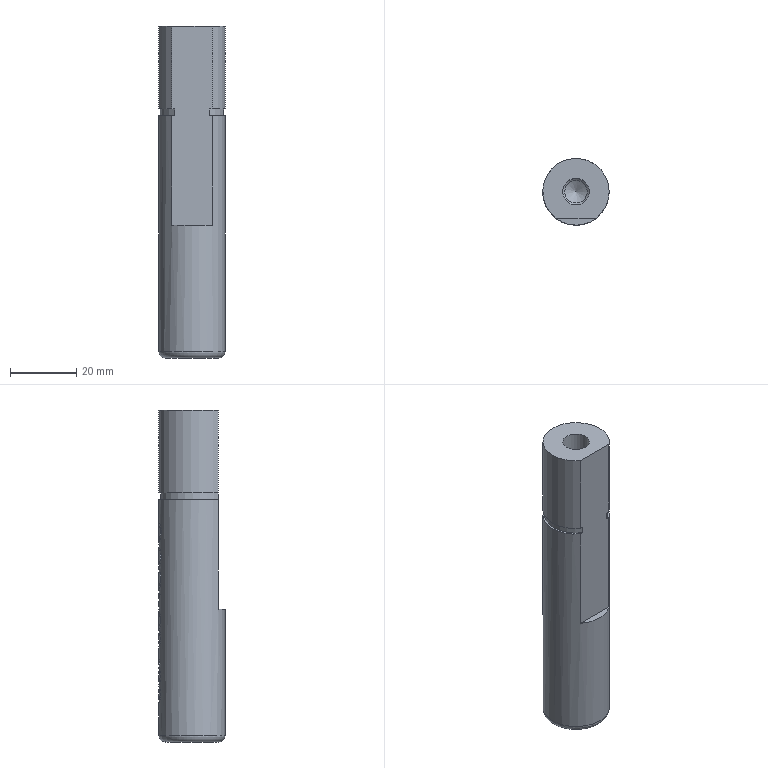Part | STEP file | PN_0061_id1870_x_t | 1 solid | 158 faces | box 20 x 20 x 100 mm | volume 29183 mm3 | plane 83 | cylinder 72 | cone 2 | torus 1 | commonest cylinder face diameters 19.8 x10 20 x7 3.205 x3 3.824 x3 3.836 x3 3.88 x3